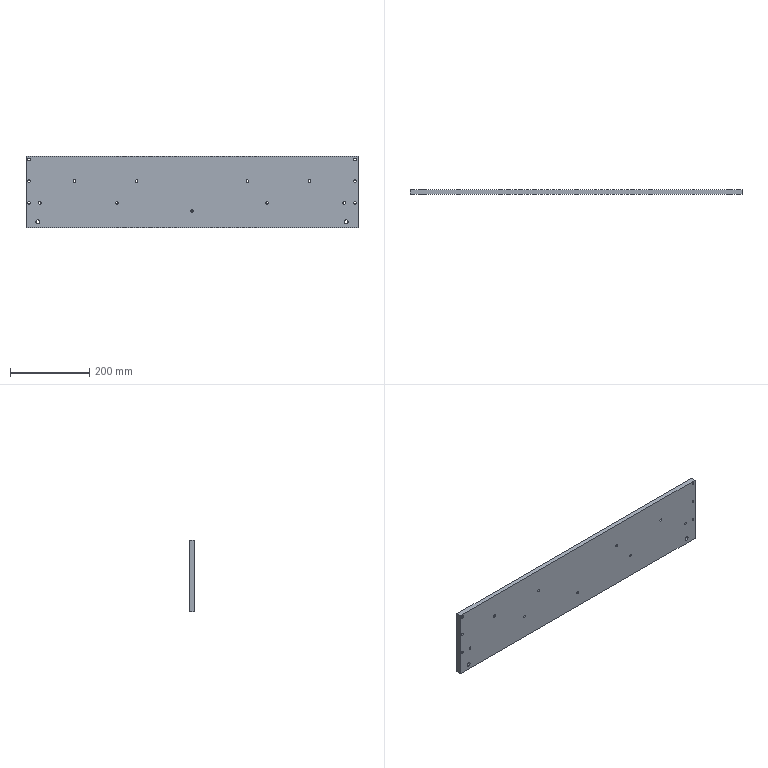Part | STEP file | 0244_217_Plate | 1 solid | 40 faces | box 840 x 12 x 180 mm | volume 1806542 mm3 | cylinder 34 | plane 6 | commonest cylinder face diameters 6.5 x30 10 x4